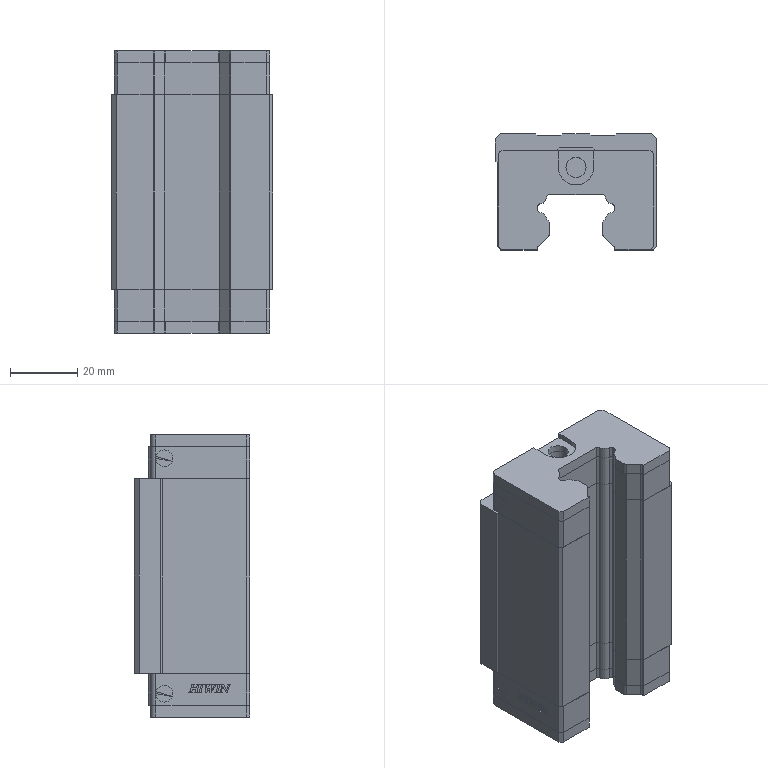Part | SolidWorks | features BaseBody 5 | 5 solids | 544 faces | box 48 x 34.5 x 84 mm | volume 102162 mm3 | plane 384 | cylinder 148 | cone 12 | commonest cylinder face diameters 2 x20 4.6 x20 0.207 x17 0.24 x17 0.104 x9 0.12 x9